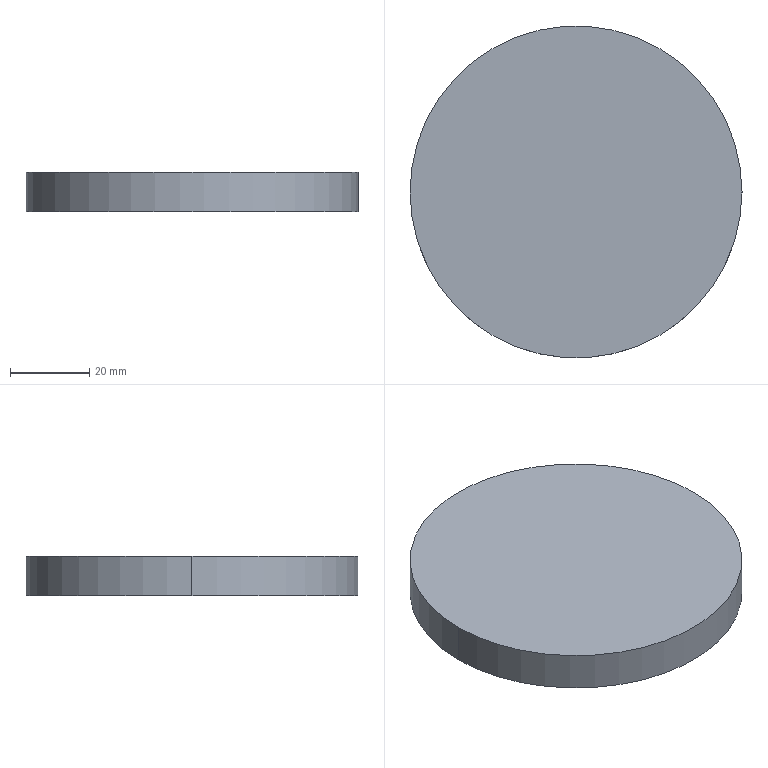Part | SolidWorks | features Extrusion 1 | 1 solid | 4 faces | box 84 x 84 x 10 mm | volume 55418 mm3 | cylinder 2 | plane 2 | commonest cylinder face diameters 84 x2
STEP:
#1=CARTESIAN_POINT('',(42.,0.,-5.));
#2=VERTEX_POINT('',#1);
#3=CARTESIAN_POINT('',(-42.,0.,-5.));
#4=VERTEX_POINT('',#3);
#5=CARTESIAN_POINT('',(0.,0.,-5.));
#6=DIRECTION('',(0.,0.,1.));
#7=DIRECTION('',(1.,0.,0.));
#8=AXIS2_PLACEMENT_3D('',#5,#6,#7);
#9=CIRCLE('',#8,42.);
#10=EDGE_CURVE('',#2,#4,#9,.T.);
#11=ORIENTED_EDGE('',*,*,#10,.T.);
#12=CARTESIAN_POINT('',(-42.,0.,5.));
#13=VERTEX_POINT('',#12);
#14=CARTESIAN_POINT('',(-42.,0.,-5.));
#15=DIRECTION('',(0.,0.,1.));
#16=VECTOR('',#15,1000.);
#17=LINE('',#14,#16);
#18=EDGE_CURVE('',#4,#13,#17,.T.);
#19=ORIENTED_EDGE('',*,*,#18,.T.);
#20=CARTESIAN_POINT('',(42.,0.,5.));
#21=VERTEX_POINT('',#20);
#22=CARTESIAN_POINT('',(0.,0.,5.));
#23=DIRECTION('',(0.,0.,1.));
#24=DIRECTION('',(1.,0.,0.));
#25=AXIS2_PLACEMENT_3D('',#22,#23,#24);
#26=CIRCLE('',#25,42.);
#27=EDGE_CURVE('',#21,#13,#26,.T.);
#28=ORIENTED_EDGE('',*,*,#27,.F.);
#29=CARTESIAN_POINT('',(42.,0.,-5.));
#30=DIRECTION('',(0.,0.,1.));
#31=VECTOR('',#30,1000.);
#32=LINE('',#29,#31);
#33=EDGE_CURVE('',#2,#21,#32,.T.);
#34=ORIENTED_EDGE('',*,*,#33,.F.);
#35=EDGE_LOOP('',(#11,#19,#28,#34));
#36=FACE_OUTER_BOUND('',#35,.T.);
#37=CARTESIAN_POINT('',(0.,0.,-5.));
#38=DIRECTION('',(0.,0.,1.));
#39=DIRECTION('',(1.,0.,0.));
#40=AXIS2_PLACEMENT_3D('',#37,#38,#39);
#41=CYLINDRICAL_SURFACE('',#40,42.);
#42=ADVANCED_FACE('',(#36),#41,.T.);
#43=ORIENTED_EDGE('',*,*,#18,.F.);
#44=CARTESIAN_POINT('',(0.,0.,-5.));
#45=DIRECTION('',(0.,0.,1.));
#46=DIRECTION('',(1.,0.,0.));
#47=AXIS2_PLACEMENT_3D('',#44,#45,#46);
#48=CIRCLE('',#47,42.);
#49=EDGE_CURVE('',#4,#2,#48,.T.);
#50=ORIENTED_EDGE('',*,*,#49,.T.);
#51=ORIENTED_EDGE('',*,*,#33,.T.);
#52=CARTESIAN_POINT('',(0.,0.,5.));
#53=DIRECTION('',(0.,0.,1.));
#54=DIRECTION('',(1.,0.,0.));
#55=AXIS2_PLACEMENT_3D('',#52,#53,#54);
#56=CIRCLE('',#55,42.);
#57=EDGE_CURVE('',#13,#21,#56,.T.);
#58=ORIENTED_EDGE('',*,*,#57,.F.);
#59=EDGE_LOOP('',(#43,#50,#51,#58));
#60=FACE_OUTER_BOUND('',#59,.T.);
#61=CARTESIAN_POINT('',(0.,0.,-5.));
#62=DIRECTION('',(0.,0.,1.));
#63=DIRECTION('',(1.,0.,0.));
#64=AXIS2_PLACEMENT_3D('',#61,#62,#63);
#65=CYLINDRICAL_SURFACE('',#64,42.);
#66=ADVANCED_FACE('',(#60),#65,.T.);
#67=ORIENTED_EDGE('',*,*,#10,.F.);
#68=ORIENTED_EDGE('',*,*,#49,.F.);
#69=EDGE_LOOP('',(#67,#68));
#70=FACE_OUTER_BOUND('',#69,.T.);
#71=CARTESIAN_POINT('',(0.,0.,-5.));
#72=DIRECTION('',(0.,0.,1.));
#73=DIRECTION('',(1.,0.,0.));
#74=AXIS2_PLACEMENT_3D('',#71,#72,#73);
#75=PLANE('',#74);
#76=ADVANCED_FACE('',(#70),#75,.F.);
#77=ORIENTED_EDGE('',*,*,#27,.T.);
#78=ORIENTED_EDGE('',*,*,#57,.T.);
#79=EDGE_LOOP('',(#77,#78));
#80=FACE_OUTER_BOUND('',#79,.T.);
#81=CARTESIAN_POINT('',(0.,0.,5.));
#82=DIRECTION('',(0.,0.,1.));
#83=DIRECTION('',(1.,0.,0.));
#84=AXIS2_PLACEMENT_3D('',#81,#82,#83);
#85=PLANE('',#84);
#86=ADVANCED_FACE('',(#80),#85,.T.);
#87=CLOSED_SHELL('',(#42,#66,#76,#86));
#88=MANIFOLD_SOLID_BREP('',#87);
#89=CARTESIAN_POINT('',(0.,0.,0.));
#90=DIRECTION('',(0.,0.,1.));
#91=DIRECTION('',(1.,0.,0.));
#92=AXIS2_PLACEMENT_3D('',#89,#90,#91);
#93=(LENGTH_UNIT()NAMED_UNIT(*)SI_UNIT(.MILLI.,.METRE.));
#94=UNCERTAINTY_MEASURE_WITH_UNIT(LENGTH_MEASURE(0.00001),#93,'','');
#95=(NAMED_UNIT(*)PLANE_ANGLE_UNIT()SI_UNIT($,.RADIAN.));
#96=(NAMED_UNIT(*)SI_UNIT($,.STERADIAN.)SOLID_ANGLE_UNIT());
#97=(GEOMETRIC_REPRESENTATION_CONTEXT(3)GLOBAL_UNCERTAINTY_ASSIGNED_CONTEXT((#94))GLOBAL_UNIT_ASSIGNED_CONTEXT((#93,#95,#96))REPRESENTATION_CONTEXT('',''));
#98=ADVANCED_BREP_SHAPE_REPRESENTATION('',(#88,#92),#97);